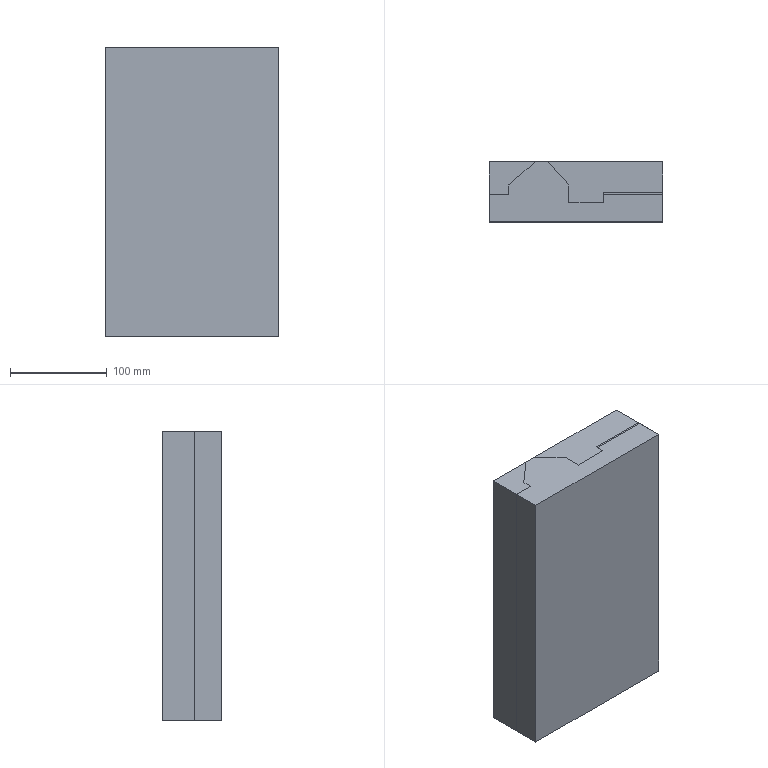Part | NX | 3 solids | 34 faces | box 180 x 62 x 300 mm | volume 7148100 mm3 | plane 34
STEP:
#1=CARTESIAN_POINT('',(-90.,31.,300.));
#2=VERTEX_POINT('',#1);
#3=CARTESIAN_POINT('',(-90.,31.,0.));
#4=VERTEX_POINT('',#3);
#5=CARTESIAN_POINT('',(-90.,31.,150.));
#6=DIRECTION('',(0.,0.,-1.));
#7=VECTOR('',#6,1000.);
#8=LINE('',#5,#7);
#9=EDGE_CURVE('',#2,#4,#8,.T.);
#10=ORIENTED_EDGE('',*,*,#9,.F.);
#11=CARTESIAN_POINT('',(90.,31.,300.));
#12=VERTEX_POINT('',#11);
#13=CARTESIAN_POINT('',(0.,31.,300.));
#14=DIRECTION('',(-1.,0.,0.));
#15=VECTOR('',#14,1000.);
#16=LINE('',#13,#15);
#17=EDGE_CURVE('',#12,#2,#16,.T.);
#18=ORIENTED_EDGE('',*,*,#17,.F.);
#19=CARTESIAN_POINT('',(90.,31.,0.));
#20=VERTEX_POINT('',#19);
#21=CARTESIAN_POINT('',(90.,31.,150.));
#22=DIRECTION('',(0.,0.,1.));
#23=VECTOR('',#22,1000.);
#24=LINE('',#21,#23);
#25=EDGE_CURVE('',#20,#12,#24,.T.);
#26=ORIENTED_EDGE('',*,*,#25,.F.);
#27=CARTESIAN_POINT('',(0.,31.,0.));
#28=DIRECTION('',(1.,0.,0.));
#29=VECTOR('',#28,1000.);
#30=LINE('',#27,#29);
#31=EDGE_CURVE('',#4,#20,#30,.T.);
#32=ORIENTED_EDGE('',*,*,#31,.F.);
#33=EDGE_LOOP('',(#10,#18,#26,#32));
#34=FACE_BOUND('',#33,.T.);
#35=CARTESIAN_POINT('',(0.,31.,150.));
#36=DIRECTION('',(0.,1.,0.));
#37=DIRECTION('',(0.,0.,1.));
#38=AXIS2_PLACEMENT_3D('',#35,#36,#37);
#39=PLANE('',#38);
#40=ADVANCED_FACE('',(#34),#39,.T.);
#41=CARTESIAN_POINT('',(-90.,-31.,300.));
#42=VERTEX_POINT('',#41);
#43=CARTESIAN_POINT('',(-90.,-31.,300.));
#44=DIRECTION('',(0.,1.,0.));
#45=VECTOR('',#44,1000.);
#46=LINE('',#43,#45);
#47=EDGE_CURVE('',#42,#2,#46,.T.);
#48=ORIENTED_EDGE('',*,*,#47,.T.);
#49=ORIENTED_EDGE('',*,*,#9,.T.);
#50=CARTESIAN_POINT('',(-90.,-31.,0.));
#51=VERTEX_POINT('',#50);
#52=CARTESIAN_POINT('',(-90.,-31.,0.));
#53=DIRECTION('',(0.,1.,0.));
#54=VECTOR('',#53,1000.);
#55=LINE('',#52,#54);
#56=EDGE_CURVE('',#51,#4,#55,.T.);
#57=ORIENTED_EDGE('',*,*,#56,.F.);
#58=CARTESIAN_POINT('',(-90.,-31.,150.));
#59=DIRECTION('',(0.,0.,1.));
#60=VECTOR('',#59,1000.);
#61=LINE('',#58,#60);
#62=EDGE_CURVE('',#51,#42,#61,.T.);
#63=ORIENTED_EDGE('',*,*,#62,.T.);
#64=EDGE_LOOP('',(#48,#49,#57,#63));
#65=FACE_BOUND('',#64,.T.);
#66=CARTESIAN_POINT('',(-90.,-31.,150.));
#67=DIRECTION('',(-1.,0.,0.));
#68=DIRECTION('',(0.,-1.,0.));
#69=AXIS2_PLACEMENT_3D('',#66,#67,#68);
#70=PLANE('',#69);
#71=ADVANCED_FACE('',(#65),#70,.T.);
#72=ORIENTED_EDGE('',*,*,#56,.T.);
#73=ORIENTED_EDGE('',*,*,#31,.T.);
#74=CARTESIAN_POINT('',(90.,-31.,0.));
#75=VERTEX_POINT('',#74);
#76=CARTESIAN_POINT('',(90.,-31.,0.));
#77=DIRECTION('',(0.,1.,0.));
#78=VECTOR('',#77,1000.);
#79=LINE('',#76,#78);
#80=EDGE_CURVE('',#75,#20,#79,.T.);
#81=ORIENTED_EDGE('',*,*,#80,.F.);
#82=CARTESIAN_POINT('',(0.,-31.,0.));
#83=DIRECTION('',(-1.,0.,0.));
#84=VECTOR('',#83,1000.);
#85=LINE('',#82,#84);
#86=EDGE_CURVE('',#75,#51,#85,.T.);
#87=ORIENTED_EDGE('',*,*,#86,.T.);
#88=EDGE_LOOP('',(#72,#73,#81,#87));
#89=FACE_BOUND('',#88,.T.);
#90=CARTESIAN_POINT('',(0.,-31.,0.));
#91=DIRECTION('',(0.,0.,-1.));
#92=DIRECTION('',(0.,1.,0.));
#93=AXIS2_PLACEMENT_3D('',#90,#91,#92);
#94=PLANE('',#93);
#95=ADVANCED_FACE('',(#89),#94,.T.);
#96=ORIENTED_EDGE('',*,*,#80,.T.);
#97=ORIENTED_EDGE('',*,*,#25,.T.);
#98=CARTESIAN_POINT('',(90.,-31.,300.));
#99=VERTEX_POINT('',#98);
#100=CARTESIAN_POINT('',(90.,-31.,300.));
#101=DIRECTION('',(0.,1.,0.));
#102=VECTOR('',#101,1000.);
#103=LINE('',#100,#102);
#104=EDGE_CURVE('',#99,#12,#103,.T.);
#105=ORIENTED_EDGE('',*,*,#104,.F.);
#106=CARTESIAN_POINT('',(90.,-31.,150.));
#107=DIRECTION('',(0.,0.,-1.));
#108=VECTOR('',#107,1000.);
#109=LINE('',#106,#108);
#110=EDGE_CURVE('',#99,#75,#109,.T.);
#111=ORIENTED_EDGE('',*,*,#110,.T.);
#112=EDGE_LOOP('',(#96,#97,#105,#111));
#113=FACE_BOUND('',#112,.T.);
#114=CARTESIAN_POINT('',(90.,-31.,150.));
#115=DIRECTION('',(1.,0.,0.));
#116=DIRECTION('',(0.,1.,0.));
#117=AXIS2_PLACEMENT_3D('',#114,#115,#116);
#118=PLANE('',#117);
#119=ADVANCED_FACE('',(#113),#118,.T.);
#120=CARTESIAN_POINT('',(0.,-31.,300.));
#121=DIRECTION('',(1.,0.,0.));
#122=VECTOR('',#121,1000.);
#123=LINE('',#120,#122);
#124=EDGE_CURVE('',#42,#99,#123,.T.);
#125=ORIENTED_EDGE('',*,*,#124,.F.);
#126=ORIENTED_EDGE('',*,*,#62,.F.);
#127=ORIENTED_EDGE('',*,*,#86,.F.);
#128=ORIENTED_EDGE('',*,*,#110,.F.);
#129=EDGE_LOOP('',(#125,#126,#127,#128));
#130=FACE_BOUND('',#129,.T.);
#131=CARTESIAN_POINT('',(0.,-31.,150.));
#132=DIRECTION('',(0.,-1.,0.));
#133=DIRECTION('',(0.,0.,-1.));
#134=AXIS2_PLACEMENT_3D('',#131,#132,#133);
#135=PLANE('',#134);
#136=ADVANCED_FACE('',(#130),#135,.T.);
#137=ORIENTED_EDGE('',*,*,#124,.T.);
#138=ORIENTED_EDGE('',*,*,#104,.T.);
#139=ORIENTED_EDGE('',*,*,#17,.T.);
#140=ORIENTED_EDGE('',*,*,#47,.F.);
#141=EDGE_LOOP('',(#137,#138,#139,#140));
#142=FACE_BOUND('',#141,.T.);
#143=CARTESIAN_POINT('',(0.,-31.,300.));
#144=DIRECTION('',(0.,0.,1.));
#145=DIRECTION('',(0.,-1.,0.));
#146=AXIS2_PLACEMENT_3D('',#143,#144,#145);
#147=PLANE('',#146);
#148=ADVANCED_FACE('',(#142),#147,.T.);
#149=CLOSED_SHELL('',(#40,#71,#95,#119,#136,#148));
#150=MANIFOLD_SOLID_BREP('',#149);
#151=CARTESIAN_POINT('',(-69.5,7.,0.));
#152=VERTEX_POINT('',#151);
#153=CARTESIAN_POINT('',(-42.372,31.,0.));
#154=VERTEX_POINT('',#153);
#155=CARTESIAN_POINT('',(-69.5,7.,0.));
#156=DIRECTION('',(0.749,0.6626,0.));
#157=VECTOR('',#156,1000.);
#158=LINE('',#155,#157);
#159=EDGE_CURVE('',#152,#154,#158,.T.);
#160=ORIENTED_EDGE('',*,*,#159,.F.);
#161=CARTESIAN_POINT('',(-69.5,7.,300.));
#162=VERTEX_POINT('',#161);
#163=CARTESIAN_POINT('',(-69.5,7.,300.));
#164=DIRECTION('',(0.,0.,-1.));
#165=VECTOR('',#164,1000.);
#166=LINE('',#163,#165);
#167=EDGE_CURVE('',#162,#152,#166,.T.);
#168=ORIENTED_EDGE('',*,*,#167,.F.);
#169=CARTESIAN_POINT('',(-42.372,31.,300.));
#170=VERTEX_POINT('',#169);
#171=CARTESIAN_POINT('',(-69.5,7.,300.));
#172=DIRECTION('',(0.749,0.6626,0.));
#173=VECTOR('',#172,1000.);
#174=LINE('',#171,#173);
#175=EDGE_CURVE('',#162,#170,#174,.T.);
#176=ORIENTED_EDGE('',*,*,#175,.T.);
#177=CARTESIAN_POINT('',(-42.372,31.,300.));
#178=DIRECTION('',(0.,0.,-1.));
#179=VECTOR('',#178,1000.);
#180=LINE('',#177,#179);
#181=EDGE_CURVE('',#170,#154,#180,.T.);
#182=ORIENTED_EDGE('',*,*,#181,.T.);
#183=EDGE_LOOP('',(#160,#168,#176,#182));
#184=FACE_BOUND('',#183,.T.);
#185=CARTESIAN_POINT('',(-69.5,7.,300.));
#186=DIRECTION('',(-0.6626,0.749,0.));
#187=DIRECTION('',(-0.749,-0.6626,0.));
#188=AXIS2_PLACEMENT_3D('',#185,#186,#187);
#189=PLANE('',#188);
#190=ADVANCED_FACE('',(#184),#189,.T.);
#191=CARTESIAN_POINT('',(-29.372,31.,0.));
#192=VERTEX_POINT('',#191);
#193=CARTESIAN_POINT('',(-42.372,31.,0.));
#194=DIRECTION('',(1.,0.,0.));
#195=VECTOR('',#194,1000.);
#196=LINE('',#193,#195);
#197=EDGE_CURVE('',#154,#192,#196,.T.);
#198=ORIENTED_EDGE('',*,*,#197,.F.);
#199=ORIENTED_EDGE('',*,*,#181,.F.);
#200=CARTESIAN_POINT('',(-29.372,31.,300.));
#201=VERTEX_POINT('',#200);
#202=CARTESIAN_POINT('',(-42.372,31.,300.));
#203=DIRECTION('',(1.,0.,0.));
#204=VECTOR('',#203,1000.);
#205=LINE('',#202,#204);
#206=EDGE_CURVE('',#170,#201,#205,.T.);
#207=ORIENTED_EDGE('',*,*,#206,.T.);
#208=CARTESIAN_POINT('',(-29.372,31.,300.));
#209=DIRECTION('',(0.,0.,-1.));
#210=VECTOR('',#209,1000.);
#211=LINE('',#208,#210);
#212=EDGE_CURVE('',#201,#192,#211,.T.);
#213=ORIENTED_EDGE('',*,*,#212,.T.);
#214=EDGE_LOOP('',(#198,#199,#207,#213));
#215=FACE_BOUND('',#214,.T.);
#216=CARTESIAN_POINT('',(-42.372,31.,300.));
#217=DIRECTION('',(0.,1.,0.));
#218=DIRECTION('',(0.,0.,1.));
#219=AXIS2_PLACEMENT_3D('',#216,#217,#218);
#220=PLANE('',#219);
#221=ADVANCED_FACE('',(#215),#220,.T.);
#222=CARTESIAN_POINT('',(-7.5,7.,0.));
#223=VERTEX_POINT('',#222);
#224=CARTESIAN_POINT('',(-29.372,31.,0.));
#225=DIRECTION('',(0.6736,-0.7391,0.));
#226=VECTOR('',#225,1000.);
#227=LINE('',#224,#226);
#228=EDGE_CURVE('',#192,#223,#227,.T.);
#229=ORIENTED_EDGE('',*,*,#228,.F.);
#230=ORIENTED_EDGE('',*,*,#212,.F.);
#231=CARTESIAN_POINT('',(-7.5,7.,300.));
#232=VERTEX_POINT('',#231);
#233=CARTESIAN_POINT('',(-29.372,31.,300.));
#234=DIRECTION('',(0.6736,-0.7391,0.));
#235=VECTOR('',#234,1000.);
#236=LINE('',#233,#235);
#237=EDGE_CURVE('',#201,#232,#236,.T.);
#238=ORIENTED_EDGE('',*,*,#237,.T.);
#239=CARTESIAN_POINT('',(-7.5,7.,300.));
#240=DIRECTION('',(0.,0.,-1.));
#241=VECTOR('',#240,1000.);
#242=LINE('',#239,#241);
#243=EDGE_CURVE('',#232,#223,#242,.T.);
#244=ORIENTED_EDGE('',*,*,#243,.T.);
#245=EDGE_LOOP('',(#229,#230,#238,#244));
#246=FACE_BOUND('',#245,.T.);
#247=CARTESIAN_POINT('',(-29.372,31.,300.));
#248=DIRECTION('',(0.7391,0.6736,0.));
#249=DIRECTION('',(-0.6736,0.7391,0.));
#250=AXIS2_PLACEMENT_3D('',#247,#248,#249);
#251=PLANE('',#250);
#252=ADVANCED_FACE('',(#246),#251,.T.);
#253=CARTESIAN_POINT('',(-7.5,-11.,0.));
#254=VERTEX_POINT('',#253);
#255=CARTESIAN_POINT('',(-7.5,-3.,0.));
#256=DIRECTION('',(0.,-1.,0.));
#257=VECTOR('',#256,1000.);
#258=LINE('',#255,#257);
#259=EDGE_CURVE('',#223,#254,#258,.T.);
#260=ORIENTED_EDGE('',*,*,#259,.F.);
#261=ORIENTED_EDGE('',*,*,#243,.F.);
#262=CARTESIAN_POINT('',(-7.5,-11.,300.));
#263=VERTEX_POINT('',#262);
#264=CARTESIAN_POINT('',(-7.5,7.,300.));
#265=DIRECTION('',(0.,-1.,0.));
#266=VECTOR('',#265,1000.);
#267=LINE('',#264,#266);
#268=EDGE_CURVE('',#232,#263,#267,.T.);
#269=ORIENTED_EDGE('',*,*,#268,.T.);
#270=CARTESIAN_POINT('',(-7.5,-11.,300.));
#271=DIRECTION('',(0.,0.,-1.));
#272=VECTOR('',#271,1000.);
#273=LINE('',#270,#272);
#274=EDGE_CURVE('',#263,#254,#273,.T.);
#275=ORIENTED_EDGE('',*,*,#274,.T.);
#276=EDGE_LOOP('',(#260,#261,#269,#275));
#277=FACE_BOUND('',#276,.T.);
#278=CARTESIAN_POINT('',(-7.5,-3.,300.));
#279=DIRECTION('',(1.,0.,0.));
#280=DIRECTION('',(0.,0.,-1.));
#281=AXIS2_PLACEMENT_3D('',#278,#279,#280);
#282=PLANE('',#281);
#283=ADVANCED_FACE('',(#277),#282,.T.);
#284=CARTESIAN_POINT('',(28.5,-11.,0.));
#285=VERTEX_POINT('',#284);
#286=CARTESIAN_POINT('',(-7.5,-11.,0.));
#287=DIRECTION('',(1.,0.,0.));
#288=VECTOR('',#287,1000.);
#289=LINE('',#286,#288);
#290=EDGE_CURVE('',#254,#285,#289,.T.);
#291=ORIENTED_EDGE('',*,*,#290,.F.);
#292=ORIENTED_EDGE('',*,*,#274,.F.);
#293=CARTESIAN_POINT('',(28.5,-11.,300.));
#294=VERTEX_POINT('',#293);
#295=CARTESIAN_POINT('',(-7.5,-11.,300.));
#296=DIRECTION('',(1.,0.,0.));
#297=VECTOR('',#296,1000.);
#298=LINE('',#295,#297);
#299=EDGE_CURVE('',#263,#294,#298,.T.);
#300=ORIENTED_EDGE('',*,*,#299,.T.);
#301=CARTESIAN_POINT('',(28.5,-11.,300.));
#302=DIRECTION('',(0.,0.,-1.));
#303=VECTOR('',#302,1000.);
#304=LINE('',#301,#303);
#305=EDGE_CURVE('',#294,#285,#304,.T.);
#306=ORIENTED_EDGE('',*,*,#305,.T.);
#307=EDGE_LOOP('',(#291,#292,#300,#306));
#308=FACE_BOUND('',#307,.T.);
#309=CARTESIAN_POINT('',(-7.5,-11.,300.));
#310=DIRECTION('',(0.,1.,0.));
#311=DIRECTION('',(-1.,0.,0.));
#312=AXIS2_PLACEMENT_3D('',#309,#310,#311);
#313=PLANE('',#312);
#314=ADVANCED_FACE('',(#308),#313,.T.);
#315=CARTESIAN_POINT('',(28.5,-1.,0.));
#316=VERTEX_POINT('',#315);
#317=CARTESIAN_POINT('',(28.5,-11.,0.));
#318=DIRECTION('',(0.,1.,0.));
#319=VECTOR('',#318,1000.);
#320=LINE('',#317,#319);
#321=EDGE_CURVE('',#285,#316,#320,.T.);
#322=ORIENTED_EDGE('',*,*,#321,.F.);
#323=ORIENTED_EDGE('',*,*,#305,.F.);
#324=CARTESIAN_POINT('',(28.5,-1.,300.));
#325=VERTEX_POINT('',#324);
#326=CARTESIAN_POINT('',(28.5,-11.,300.));
#327=DIRECTION('',(0.,1.,0.));
#328=VECTOR('',#327,1000.);
#329=LINE('',#326,#328);
#330=EDGE_CURVE('',#294,#325,#329,.T.);
#331=ORIENTED_EDGE('',*,*,#330,.T.);
#332=CARTESIAN_POINT('',(28.5,-1.,300.));
#333=DIRECTION('',(0.,0.,-1.));
#334=VECTOR('',#333,1000.);
#335=LINE('',#332,#334);
#336=EDGE_CURVE('',#325,#316,#335,.T.);
#337=ORIENTED_EDGE('',*,*,#336,.T.);
#338=EDGE_LOOP('',(#322,#323,#331,#337));
#339=FACE_BOUND('',#338,.T.);
#340=CARTESIAN_POINT('',(28.5,-11.,300.));
#341=DIRECTION('',(-1.,0.,0.));
#342=DIRECTION('',(0.,0.,1.));
#343=AXIS2_PLACEMENT_3D('',#340,#341,#342);
#344=PLANE('',#343);
#345=ADVANCED_FACE('',(#339),#344,.T.);
#346=CARTESIAN_POINT('',(90.,-1.,0.));
#347=VERTEX_POINT('',#346);
#348=CARTESIAN_POINT('',(0.,-1.,0.));
#349=DIRECTION('',(1.,0.,0.));
#350=VECTOR('',#349,1000.);
#351=LINE('',#348,#350);
#352=EDGE_CURVE('',#316,#347,#351,.T.);
#353=ORIENTED_EDGE('',*,*,#352,.F.);
#354=ORIENTED_EDGE('',*,*,#336,.F.);
#355=CARTESIAN_POINT('',(90.,-1.,300.));
#356=VERTEX_POINT('',#355);
#357=CARTESIAN_POINT('',(0.,-1.,300.));
#358=DIRECTION('',(1.,0.,0.));
#359=VECTOR('',#358,1000.);
#360=LINE('',#357,#359);
#361=EDGE_CURVE('',#325,#356,#360,.T.);
#362=ORIENTED_EDGE('',*,*,#361,.T.);
#363=CARTESIAN_POINT('',(90.,-1.,300.));
#364=DIRECTION('',(0.,0.,-1.));
#365=VECTOR('',#364,1000.);
#366=LINE('',#363,#365);
#367=EDGE_CURVE('',#356,#347,#366,.T.);
#368=ORIENTED_EDGE('',*,*,#367,.T.);
#369=EDGE_LOOP('',(#353,#354,#362,#368));
#370=FACE_BOUND('',#369,.T.);
#371=CARTESIAN_POINT('',(28.5,-1.,300.));
#372=DIRECTION('',(0.,1.,0.));
#373=DIRECTION('',(-1.,0.,0.));
#374=AXIS2_PLACEMENT_3D('',#371,#372,#373);
#375=PLANE('',#374);
#376=ADVANCED_FACE('',(#370),#375,.T.);
#377=CARTESIAN_POINT('',(90.,-31.,0.));
#378=VERTEX_POINT('',#377);
#379=CARTESIAN_POINT('',(90.,0.,0.));
#380=DIRECTION('',(0.,-1.,0.));
#381=VECTOR('',#380,1000.);
#382=LINE('',#379,#381);
#383=EDGE_CURVE('',#347,#378,#382,.T.);
#384=ORIENTED_EDGE('',*,*,#383,.F.);
#385=ORIENTED_EDGE('',*,*,#367,.F.);
#386=CARTESIAN_POINT('',(90.,-31.,300.));
#387=VERTEX_POINT('',#386);
#388=CARTESIAN_POINT('',(90.,0.,300.));
#389=DIRECTION('',(0.,-1.,0.));
#390=VECTOR('',#389,1000.);
#391=LINE('',#388,#390);
#392=EDGE_CURVE('',#356,#387,#391,.T.);
#393=ORIENTED_EDGE('',*,*,#392,.T.);
#394=CARTESIAN_POINT('',(90.,-31.,300.));
#395=DIRECTION('',(0.,0.,-1.));
#396=VECTOR('',#395,1000.);
#397=LINE('',#394,#396);
#398=EDGE_CURVE('',#387,#378,#397,.T.);
#399=ORIENTED_EDGE('',*,*,#398,.T.);
#400=EDGE_LOOP('',(#384,#385,#393,#399));
#401=FACE_BOUND('',#400,.T.);
#402=CARTESIAN_POINT('',(90.,-3.,300.));
#403=DIRECTION('',(1.,0.,0.));
#404=DIRECTION('',(0.,1.,0.));
#405=AXIS2_PLACEMENT_3D('',#402,#403,#404);
#406=PLANE('',#405);
#407=ADVANCED_FACE('',(#401),#406,.T.);
#408=CARTESIAN_POINT('',(-90.,-31.,0.));
#409=VERTEX_POINT('',#408);
#410=CARTESIAN_POINT('',(90.5,-31.,0.));
#411=DIRECTION('',(-1.,0.,0.));
#412=VECTOR('',#411,1000.);
#413=LINE('',#410,#412);
#414=EDGE_CURVE('',#378,#409,#413,.T.);
#415=ORIENTED_EDGE('',*,*,#414,.F.);
#416=ORIENTED_EDGE('',*,*,#398,.F.);
#417=CARTESIAN_POINT('',(-90.,-31.,300.));
#418=VERTEX_POINT('',#417);
#419=CARTESIAN_POINT('',(90.5,-31.,300.));
#420=DIRECTION('',(-1.,0.,0.));
#421=VECTOR('',#420,1000.);
#422=LINE('',#419,#421);
#423=EDGE_CURVE('',#387,#418,#422,.T.);
#424=ORIENTED_EDGE('',*,*,#423,.T.);
#425=CARTESIAN_POINT('',(-90.,-31.,300.));
#426=DIRECTION('',(0.,0.,-1.));
#427=VECTOR('',#426,1000.);
#428=LINE('',#425,#427);
#429=EDGE_CURVE('',#418,#409,#428,.T.);
#430=ORIENTED_EDGE('',*,*,#429,.T.);
#431=EDGE_LOOP('',(#415,#416,#424,#430));
#432=FACE_BOUND('',#431,.T.);
#433=CARTESIAN_POINT('',(90.5,-31.,300.));
#434=DIRECTION('',(0.,-1.,0.));
#435=DIRECTION('',(0.,0.,-1.));
#436=AXIS2_PLACEMENT_3D('',#433,#434,#435);
#437=PLANE('',#436);
#438=ADVANCED_FACE('',(#432),#437,.T.);
#439=CARTESIAN_POINT('',(-90.,-3.,0.));
#440=VERTEX_POINT('',#439);
#441=CARTESIAN_POINT('',(-90.,0.,0.));
#442=DIRECTION('',(0.,1.,0.));
#443=VECTOR('',#442,1000.);
#444=LINE('',#441,#443);
#445=EDGE_CURVE('',#409,#440,#444,.T.);
#446=ORIENTED_EDGE('',*,*,#445,.F.);
#447=ORIENTED_EDGE('',*,*,#429,.F.);
#448=CARTESIAN_POINT('',(-90.,-3.,300.));
#449=VERTEX_POINT('',#448);
#450=CARTESIAN_POINT('',(-90.,0.,300.));
#451=DIRECTION('',(0.,1.,0.));
#452=VECTOR('',#451,1000.);
#453=LINE('',#450,#452);
#454=EDGE_CURVE('',#418,#449,#453,.T.);
#455=ORIENTED_EDGE('',*,*,#454,.T.);
#456=CARTESIAN_POINT('',(-90.,-3.,300.));
#457=DIRECTION('',(0.,0.,-1.));
#458=VECTOR('',#457,1000.);
#459=LINE('',#456,#458);
#460=EDGE_CURVE('',#449,#440,#459,.T.);
#461=ORIENTED_EDGE('',*,*,#460,.T.);
#462=EDGE_LOOP('',(#446,#447,#455,#461));
#463=FACE_BOUND('',#462,.T.);
#464=CARTESIAN_POINT('',(-90.,-31.,300.));
#465=DIRECTION('',(-1.,0.,0.));
#466=DIRECTION('',(0.,-1.,0.));
#467=AXIS2_PLACEMENT_3D('',#464,#465,#466);
#468=PLANE('',#467);
#469=ADVANCED_FACE('',(#463),#468,.T.);
#470=CARTESIAN_POINT('',(-69.5,-3.,0.));
#471=VERTEX_POINT('',#470);
#472=CARTESIAN_POINT('',(-90.5,-3.,0.));
#473=DIRECTION('',(1.,0.,0.));
#474=VECTOR('',#473,1000.);
#475=LINE('',#472,#474);
#476=EDGE_CURVE('',#440,#471,#475,.T.);
#477=ORIENTED_EDGE('',*,*,#476,.F.);
#478=ORIENTED_EDGE('',*,*,#460,.F.);
#479=CARTESIAN_POINT('',(-69.5,-3.,300.));
#480=VERTEX_POINT('',#479);
#481=CARTESIAN_POINT('',(-90.5,-3.,300.));
#482=DIRECTION('',(1.,0.,0.));
#483=VECTOR('',#482,1000.);
#484=LINE('',#481,#483);
#485=EDGE_CURVE('',#449,#480,#484,.T.);
#486=ORIENTED_EDGE('',*,*,#485,.T.);
#487=CARTESIAN_POINT('',(-69.5,-3.,300.));
#488=DIRECTION('',(0.,0.,-1.));
#489=VECTOR('',#488,1000.);
#490=LINE('',#487,#489);
#491=EDGE_CURVE('',#480,#471,#490,.T.);
#492=ORIENTED_EDGE('',*,*,#491,.T.);
#493=EDGE_LOOP('',(#477,#478,#486,#492));
#494=FACE_BOUND('',#493,.T.);
#495=CARTESIAN_POINT('',(-90.5,-3.,300.));
#496=DIRECTION('',(0.,1.,0.));
#497=DIRECTION('',(0.,0.,1.));
#498=AXIS2_PLACEMENT_3D('',#495,#496,#497);
#499=PLANE('',#498);
#500=ADVANCED_FACE('',(#494),#499,.T.);
#501=CARTESIAN_POINT('',(-69.5,-3.,0.));
#502=DIRECTION('',(0.,1.,0.));
#503=VECTOR('',#502,1000.);
#504=LINE('',#501,#503);
#505=EDGE_CURVE('',#471,#152,#504,.T.);
#506=ORIENTED_EDGE('',*,*,#505,.F.);
#507=ORIENTED_EDGE('',*,*,#491,.F.);
#508=CARTESIAN_POINT('',(-69.5,-3.,300.));
#509=DIRECTION('',(0.,1.,0.));
#510=VECTOR('',#509,1000.);
#511=LINE('',#508,#510);
#512=EDGE_CURVE('',#480,#162,#511,.T.);
#513=ORIENTED_EDGE('',*,*,#512,.T.);
#514=ORIENTED_EDGE('',*,*,#167,.T.);
#515=EDGE_LOOP('',(#506,#507,#513,#514));
#516=FACE_BOUND('',#515,.T.);
#517=CARTESIAN_POINT('',(-69.5,-3.,300.));
#518=DIRECTION('',(-1.,0.,0.));
#519=DIRECTION('',(0.,0.,1.));
#520=AXIS2_PLACEMENT_3D('',#517,#518,#519);
#521=PLANE('',#520);
#522=ADVANCED_FACE('',(#516),#521,.T.);
#523=ORIENTED_EDGE('',*,*,#175,.F.);
#524=ORIENTED_EDGE('',*,*,#512,.F.);
#525=ORIENTED_EDGE('',*,*,#485,.F.);
#526=ORIENTED_EDGE('',*,*,#454,.F.);
#527=ORIENTED_EDGE('',*,*,#423,.F.);
#528=ORIENTED_EDGE('',*,*,#392,.F.);
#529=ORIENTED_EDGE('',*,*,#361,.F.);
#530=ORIENTED_EDGE('',*,*,#330,.F.);
#531=ORIENTED_EDGE('',*,*,#299,.F.);
#532=ORIENTED_EDGE('',*,*,#268,.F.);
#533=ORIENTED_EDGE('',*,*,#237,.F.);
#534=ORIENTED_EDGE('',*,*,#206,.F.);
#535=EDGE_LOOP('',(#523,#524,#525,#526,#527,#528,#529,#530,#531,#532,#533,#534));
#536=FACE_BOUND('',#535,.T.);
#537=CARTESIAN_POINT('',(0.,0.,300.));
#538=DIRECTION('',(0.,0.,-1.));
#539=DIRECTION('',(-1.,0.,0.));
#540=AXIS2_PLACEMENT_3D('',#537,#538,#539);
#541=PLANE('',#540);
#542=ADVANCED_FACE('',(#536),#541,.F.);
#543=ORIENTED_EDGE('',*,*,#159,.T.);
#544=ORIENTED_EDGE('',*,*,#197,.T.);
#545=ORIENTED_EDGE('',*,*,#228,.T.);
#546=ORIENTED_EDGE('',*,*,#259,.T.);
#547=ORIENTED_EDGE('',*,*,#290,.T.);
#548=ORIENTED_EDGE('',*,*,#321,.T.);
#549=ORIENTED_EDGE('',*,*,#352,.T.);
#550=ORIENTED_EDGE('',*,*,#383,.T.);
#551=ORIENTED_EDGE('',*,*,#414,.T.);
#552=ORIENTED_EDGE('',*,*,#445,.T.);
#553=ORIENTED_EDGE('',*,*,#476,.T.);
#554=ORIENTED_EDGE('',*,*,#505,.T.);
#555=EDGE_LOOP('',(#543,#544,#545,#546,#547,#548,#549,#550,#551,#552,#553,#554));
#556=FACE_BOUND('',#555,.T.);
#557=CARTESIAN_POINT('',(0.,0.,0.));
#558=DIRECTION('',(0.,0.,-1.));
#559=DIRECTION('',(-1.,0.,0.));
#560=AXIS2_PLACEMENT_3D('',#557,#558,#559);
#561=PLANE('',#560);
#562=ADVANCED_FACE('',(#556),#561,.T.);
#563=CLOSED_SHELL('',(#190,#221,#252,#283,#314,#345,#376,#407,#438,#469,#500,#522,#542,#562));
#564=MANIFOLD_SOLID_BREP('',#563);
#565=CARTESIAN_POINT('',(-69.5,7.,0.));
#566=VERTEX_POINT('',#565);
#567=CARTESIAN_POINT('',(-42.372,31.,0.));
#568=VERTEX_POINT('',#567);
#569=CARTESIAN_POINT('',(-69.5,7.,0.));
#570=DIRECTION('',(0.749,0.6626,0.));
#571=VECTOR('',#570,1000.);
#572=LINE('',#569,#571);
#573=EDGE_CURVE('',#566,#568,#572,.T.);
#574=ORIENTED_EDGE('',*,*,#573,.F.);
#575=CARTESIAN_POINT('',(-69.5,7.,300.));
#576=VERTEX_POINT('',#575);
#577=CARTESIAN_POINT('',(-69.5,7.,300.));
#578=DIRECTION('',(0.,0.,-1.));
#579=VECTOR('',#578,1000.);
#580=LINE('',#577,#579);
#581=EDGE_CURVE('',#576,#566,#580,.T.);
#582=ORIENTED_EDGE('',*,*,#581,.F.);
#583=CARTESIAN_POINT('',(-42.372,31.,300.));
#584=VERTEX_POINT('',#583);
#585=CARTESIAN_POINT('',(-69.5,7.,300.));
#586=DIRECTION('',(0.749,0.6626,0.));
#587=VECTOR('',#586,1000.);
#588=LINE('',#585,#587);
#589=EDGE_CURVE('',#576,#584,#588,.T.);
#590=ORIENTED_EDGE('',*,*,#589,.T.);
#591=CARTESIAN_POINT('',(-42.372,31.,300.));
#592=DIRECTION('',(0.,0.,-1.));
#593=VECTOR('',#592,1000.);
#594=LINE('',#591,#593);
#595=EDGE_CURVE('',#584,#568,#594,.T.);
#596=ORIENTED_EDGE('',*,*,#595,.T.);
#597=EDGE_LOOP('',(#574,#582,#590,#596));
#598=FACE_BOUND('',#597,.T.);
#599=CARTESIAN_POINT('',(-69.5,7.,300.));
#600=DIRECTION('',(-0.6626,0.749,0.));
#601=DIRECTION('',(-0.749,-0.6626,0.));
#602=AXIS2_PLACEMENT_3D('',#599,#600,#601);
#603=PLANE('',#602);
#604=ADVANCED_FACE('',(#598),#603,.T.);
#605=CARTESIAN_POINT('',(-29.372,31.,0.));
#606=VERTEX_POINT('',#605);
#607=CARTESIAN_POINT('',(-42.372,31.,0.));
#608=DIRECTION('',(1.,0.,0.));
#609=VECTOR('',#608,1000.);
#610=LINE('',#607,#609);
#611=EDGE_CURVE('',#568,#606,#610,.T.);
#612=ORIENTED_EDGE('',*,*,#611,.F.);
#613=ORIENTED_EDGE('',*,*,#595,.F.);
#614=CARTESIAN_POINT('',(-29.372,31.,300.));
#615=VERTEX_POINT('',#614);
#616=CARTESIAN_POINT('',(-42.372,31.,300.));
#617=DIRECTION('',(1.,0.,0.));
#618=VECTOR('',#617,1000.);
#619=LINE('',#616,#618);
#620=EDGE_CURVE('',#584,#615,#619,.T.);
#621=ORIENTED_EDGE('',*,*,#620,.T.);
#622=CARTESIAN_POINT('',(-29.372,31.,300.));
#623=DIRECTION('',(0.,0.,-1.));
#624=VECTOR('',#623,1000.);
#625=LINE('',#622,#624);
#626=EDGE_CURVE('',#615,#606,#625,.T.);
#627=ORIENTED_EDGE('',*,*,#626,.T.);
#628=EDGE_LOOP('',(#612,#613,#621,#627));
#629=FACE_BOUND('',#628,.T.);
#630=CARTESIAN_POINT('',(-42.372,31.,300.));
#631=DIRECTION('',(0.,1.,0.));
#632=DIRECTION('',(0.,0.,1.));
#633=AXIS2_PLACEMENT_3D('',#630,#631,#632);
#634=PLANE('',#633);
#635=ADVANCED_FACE('',(#629),#634,.T.);
#636=CARTESIAN_POINT('',(-7.5,7.,0.));
#637=VERTEX_POINT('',#636);
#638=CARTESIAN_POINT('',(-29.372,31.,0.));
#639=DIRECTION('',(0.6736,-0.7391,0.));
#640=VECTOR('',#639,1000.);
#641=LINE('',#638,#640);
#642=EDGE_CURVE('',#606,#637,#641,.T.);
#643=ORIENTED_EDGE('',*,*,#642,.F.);
#644=ORIENTED_EDGE('',*,*,#626,.F.);
#645=CARTESIAN_POINT('',(-7.5,7.,300.));
#646=VERTEX_POINT('',#645);
#647=CARTESIAN_POINT('',(-29.372,31.,300.));
#648=DIRECTION('',(0.6736,-0.7391,0.));
#649=VECTOR('',#648,1000.);
#650=LINE('',#647,#649);
#651=EDGE_CURVE('',#615,#646,#650,.T.);
#652=ORIENTED_EDGE('',*,*,#651,.T.);
#653=CARTESIAN_POINT('',(-7.5,7.,300.));
#654=DIRECTION('',(0.,0.,-1.));
#655=VECTOR('',#654,1000.);
#656=LINE('',#653,#655);
#657=EDGE_CURVE('',#646,#637,#656,.T.);
#658=ORIENTED_EDGE('',*,*,#657,.T.);
#659=EDGE_LOOP('',(#643,#644,#652,#658));
#660=FACE_BOUND('',#659,.T.);
#661=CARTESIAN_POINT('',(-29.372,31.,300.));
#662=DIRECTION('',(0.7391,0.6736,0.));
#663=DIRECTION('',(-0.6736,0.7391,0.));
#664=AXIS2_PLACEMENT_3D('',#661,#662,#663);
#665=PLANE('',#664);
#666=ADVANCED_FACE('',(#660),#665,.T.);
#667=CARTESIAN_POINT('',(-7.5,-11.,0.));
#668=VERTEX_POINT('',#667);
#669=CARTESIAN_POINT('',(-7.5,-3.,0.));
#670=DIRECTION('',(0.,-1.,0.));
#671=VECTOR('',#670,1000.);
#672=LINE('',#669,#671);
#673=EDGE_CURVE('',#637,#668,#672,.T.);
#674=ORIENTED_EDGE('',*,*,#673,.F.);
#675=ORIENTED_EDGE('',*,*,#657,.F.);
#676=CARTESIAN_POINT('',(-7.5,-11.,300.));
#677=VERTEX_POINT('',#676);
#678=CARTESIAN_POINT('',(-7.5,7.,300.));
#679=DIRECTION('',(0.,-1.,0.));
#680=VECTOR('',#679,1000.);
#681=LINE('',#678,#680);
#682=EDGE_CURVE('',#646,#677,#681,.T.);
#683=ORIENTED_EDGE('',*,*,#682,.T.);
#684=CARTESIAN_POINT('',(-7.5,-11.,300.));
#685=DIRECTION('',(0.,0.,-1.));
#686=VECTOR('',#685,1000.);
#687=LINE('',#684,#686);
#688=EDGE_CURVE('',#677,#668,#687,.T.);
#689=ORIENTED_EDGE('',*,*,#688,.T.);
#690=EDGE_LOOP('',(#674,#675,#683,#689));
#691=FACE_BOUND('',#690,.T.);
#692=CARTESIAN_POINT('',(-7.5,-3.,300.));
#693=DIRECTION('',(1.,0.,0.));
#694=DIRECTION('',(0.,0.,-1.));
#695=AXIS2_PLACEMENT_3D('',#692,#693,#694);
#696=PLANE('',#695);
#697=ADVANCED_FACE('',(#691),#696,.T.);
#698=CARTESIAN_POINT('',(28.5,-11.,0.));
#699=VERTEX_POINT('',#698);
#700=CARTESIAN_POINT('',(-7.5,-11.,0.));
#701=DIRECTION('',(1.,0.,0.));
#702=VECTOR('',#701,1000.);
#703=LINE('',#700,#702);
#704=EDGE_CURVE('',#668,#699,#703,.T.);
#705=ORIENTED_EDGE('',*,*,#704,.F.);
#706=ORIENTED_EDGE('',*,*,#688,.F.);
#707=CARTESIAN_POINT('',(28.5,-11.,300.));
#708=VERTEX_POINT('',#707);
#709=CARTESIAN_POINT('',(-7.5,-11.,300.));
#710=DIRECTION('',(1.,0.,0.));
#711=VECTOR('',#710,1000.);
#712=LINE('',#709,#711);
#713=EDGE_CURVE('',#677,#708,#712,.T.);
#714=ORIENTED_EDGE('',*,*,#713,.T.);
#715=CARTESIAN_POINT('',(28.5,-11.,300.));
#716=DIRECTION('',(0.,0.,-1.));
#717=VECTOR('',#716,1000.);
#718=LINE('',#715,#717);
#719=EDGE_CURVE('',#708,#699,#718,.T.);
#720=ORIENTED_EDGE('',*,*,#719,.T.);
#721=EDGE_LOOP('',(#705,#706,#714,#720));
#722=FACE_BOUND('',#721,.T.);
#723=CARTESIAN_POINT('',(-7.5,-11.,300.));
#724=DIRECTION('',(0.,1.,0.));
#725=DIRECTION('',(-1.,0.,0.));
#726=AXIS2_PLACEMENT_3D('',#723,#724,#725);
#727=PLANE('',#726);
#728=ADVANCED_FACE('',(#722),#727,.T.);
#729=CARTESIAN_POINT('',(28.5,-3.,0.));
#730=VERTEX_POINT('',#729);
#731=CARTESIAN_POINT('',(28.5,-11.,0.));
#732=DIRECTION('',(0.,1.,0.));
#733=VECTOR('',#732,1000.);
#734=LINE('',#731,#733);
#735=EDGE_CURVE('',#699,#730,#734,.T.);
#736=ORIENTED_EDGE('',*,*,#735,.F.);
#737=ORIENTED_EDGE('',*,*,#719,.F.);
#738=CARTESIAN_POINT('',(28.5,-3.,300.));
#739=VERTEX_POINT('',#738);
#740=CARTESIAN_POINT('',(28.5,-11.,300.));
#741=DIRECTION('',(0.,1.,0.));
#742=VECTOR('',#741,1000.);
#743=LINE('',#740,#742);
#744=EDGE_CURVE('',#708,#739,#743,.T.);
#745=ORIENTED_EDGE('',*,*,#744,.T.);
#746=CARTESIAN_POINT('',(28.5,-3.,300.));
#747=DIRECTION('',(0.,0.,-1.));
#748=VECTOR('',#747,1000.);
#749=LINE('',#746,#748);
#750=EDGE_CURVE('',#739,#730,#749,.T.);
#751=ORIENTED_EDGE('',*,*,#750,.T.);
#752=EDGE_LOOP('',(#736,#737,#745,#751));
#753=FACE_BOUND('',#752,.T.);
#754=CARTESIAN_POINT('',(28.5,-11.,300.));
#755=DIRECTION('',(-1.,0.,0.));
#756=DIRECTION('',(0.,0.,1.));
#757=AXIS2_PLACEMENT_3D('',#754,#755,#756);
#758=PLANE('',#757);
#759=ADVANCED_FACE('',(#753),#758,.T.);
#760=CARTESIAN_POINT('',(90.,-3.,0.));
#761=VERTEX_POINT('',#760);
#762=CARTESIAN_POINT('',(28.5,-3.,0.));
#763=DIRECTION('',(1.,0.,0.));
#764=VECTOR('',#763,1000.);
#765=LINE('',#762,#764);
#766=EDGE_CURVE('',#730,#761,#765,.T.);
#767=ORIENTED_EDGE('',*,*,#766,.F.);
#768=ORIENTED_EDGE('',*,*,#750,.F.);
#769=CARTESIAN_POINT('',(90.,-3.,300.));
#770=VERTEX_POINT('',#769);
#771=CARTESIAN_POINT('',(28.5,-3.,300.));
#772=DIRECTION('',(1.,0.,0.));
#773=VECTOR('',#772,1000.);
#774=LINE('',#771,#773);
#775=EDGE_CURVE('',#739,#770,#774,.T.);
#776=ORIENTED_EDGE('',*,*,#775,.T.);
#777=CARTESIAN_POINT('',(90.,-3.,300.));
#778=DIRECTION('',(0.,0.,-1.));
#779=VECTOR('',#778,1000.);
#780=LINE('',#777,#779);
#781=EDGE_CURVE('',#770,#761,#780,.T.);
#782=ORIENTED_EDGE('',*,*,#781,.T.);
#783=EDGE_LOOP('',(#767,#768,#776,#782));
#784=FACE_BOUND('',#783,.T.);
#785=CARTESIAN_POINT('',(28.5,-3.,300.));
#786=DIRECTION('',(0.,1.,0.));
#787=DIRECTION('',(-1.,0.,0.));
#788=AXIS2_PLACEMENT_3D('',#785,#786,#787);
#789=PLANE('',#788);
#790=ADVANCED_FACE('',(#784),#789,.T.);
#791=CARTESIAN_POINT('',(90.,-31.,0.));
#792=VERTEX_POINT('',#791);
#793=CARTESIAN_POINT('',(90.,0.,0.));
#794=DIRECTION('',(0.,-1.,0.));
#795=VECTOR('',#794,1000.);
#796=LINE('',#793,#795);
#797=EDGE_CURVE('',#761,#792,#796,.T.);
#798=ORIENTED_EDGE('',*,*,#797,.F.);
#799=ORIENTED_EDGE('',*,*,#781,.F.);
#800=CARTESIAN_POINT('',(90.,-31.,300.));
#801=VERTEX_POINT('',#800);
#802=CARTESIAN_POINT('',(90.,0.,300.));
#803=DIRECTION('',(0.,-1.,0.));
#804=VECTOR('',#803,1000.);
#805=LINE('',#802,#804);
#806=EDGE_CURVE('',#770,#801,#805,.T.);
#807=ORIENTED_EDGE('',*,*,#806,.T.);
#808=CARTESIAN_POINT('',(90.,-31.,300.));
#809=DIRECTION('',(0.,0.,-1.));
#810=VECTOR('',#809,1000.);
#811=LINE('',#808,#810);
#812=EDGE_CURVE('',#801,#792,#811,.T.);
#813=ORIENTED_EDGE('',*,*,#812,.T.);
#814=EDGE_LOOP('',(#798,#799,#807,#813));
#815=FACE_BOUND('',#814,.T.);
#816=CARTESIAN_POINT('',(90.,-3.,300.));
#817=DIRECTION('',(1.,0.,0.));
#818=DIRECTION('',(0.,1.,0.));
#819=AXIS2_PLACEMENT_3D('',#816,#817,#818);
#820=PLANE('',#819);
#821=ADVANCED_FACE('',(#815),#820,.T.);
#822=CARTESIAN_POINT('',(-90.,-31.,0.));
#823=VERTEX_POINT('',#822);
#824=CARTESIAN_POINT('',(90.5,-31.,0.));
#825=DIRECTION('',(-1.,0.,0.));
#826=VECTOR('',#825,1000.);
#827=LINE('',#824,#826);
#828=EDGE_CURVE('',#792,#823,#827,.T.);
#829=ORIENTED_EDGE('',*,*,#828,.F.);
#830=ORIENTED_EDGE('',*,*,#812,.F.);
#831=CARTESIAN_POINT('',(-90.,-31.,300.));
#832=VERTEX_POINT('',#831);
#833=CARTESIAN_POINT('',(90.5,-31.,300.));
#834=DIRECTION('',(-1.,0.,0.));
#835=VECTOR('',#834,1000.);
#836=LINE('',#833,#835);
#837=EDGE_CURVE('',#801,#832,#836,.T.);
#838=ORIENTED_EDGE('',*,*,#837,.T.);
#839=CARTESIAN_POINT('',(-90.,-31.,300.));
#840=DIRECTION('',(0.,0.,-1.));
#841=VECTOR('',#840,1000.);
#842=LINE('',#839,#841);
#843=EDGE_CURVE('',#832,#823,#842,.T.);
#844=ORIENTED_EDGE('',*,*,#843,.T.);
#845=EDGE_LOOP('',(#829,#830,#838,#844));
#846=FACE_BOUND('',#845,.T.);
#847=CARTESIAN_POINT('',(90.5,-31.,300.));
#848=DIRECTION('',(0.,-1.,0.));
#849=DIRECTION('',(0.,0.,-1.));
#850=AXIS2_PLACEMENT_3D('',#847,#848,#849);
#851=PLANE('',#850);
#852=ADVANCED_FACE('',(#846),#851,.T.);
#853=CARTESIAN_POINT('',(-90.,-3.,0.));
#854=VERTEX_POINT('',#853);
#855=CARTESIAN_POINT('',(-90.,0.,0.));
#856=DIRECTION('',(0.,1.,0.));
#857=VECTOR('',#856,1000.);
#858=LINE('',#855,#857);
#859=EDGE_CURVE('',#823,#854,#858,.T.);
#860=ORIENTED_EDGE('',*,*,#859,.F.);
#861=ORIENTED_EDGE('',*,*,#843,.F.);
#862=CARTESIAN_POINT('',(-90.,-3.,300.));
#863=VERTEX_POINT('',#862);
#864=CARTESIAN_POINT('',(-90.,0.,300.));
#865=DIRECTION('',(0.,1.,0.));
#866=VECTOR('',#865,1000.);
#867=LINE('',#864,#866);
#868=EDGE_CURVE('',#832,#863,#867,.T.);
#869=ORIENTED_EDGE('',*,*,#868,.T.);
#870=CARTESIAN_POINT('',(-90.,-3.,300.));
#871=DIRECTION('',(0.,0.,-1.));
#872=VECTOR('',#871,1000.);
#873=LINE('',#870,#872);
#874=EDGE_CURVE('',#863,#854,#873,.T.);
#875=ORIENTED_EDGE('',*,*,#874,.T.);
#876=EDGE_LOOP('',(#860,#861,#869,#875));
#877=FACE_BOUND('',#876,.T.);
#878=CARTESIAN_POINT('',(-90.,-31.,300.));
#879=DIRECTION('',(-1.,0.,0.));
#880=DIRECTION('',(0.,-1.,0.));
#881=AXIS2_PLACEMENT_3D('',#878,#879,#880);
#882=PLANE('',#881);
#883=ADVANCED_FACE('',(#877),#882,.T.);
#884=CARTESIAN_POINT('',(-69.5,-3.,0.));
#885=VERTEX_POINT('',#884);
#886=CARTESIAN_POINT('',(-90.5,-3.,0.));
#887=DIRECTION('',(1.,0.,0.));
#888=VECTOR('',#887,1000.);
#889=LINE('',#886,#888);
#890=EDGE_CURVE('',#854,#885,#889,.T.);
#891=ORIENTED_EDGE('',*,*,#890,.F.);
#892=ORIENTED_EDGE('',*,*,#874,.F.);
#893=CARTESIAN_POINT('',(-69.5,-3.,300.));
#894=VERTEX_POINT('',#893);
#895=CARTESIAN_POINT('',(-90.5,-3.,300.));
#896=DIRECTION('',(1.,0.,0.));
#897=VECTOR('',#896,1000.);
#898=LINE('',#895,#897);
#899=EDGE_CURVE('',#863,#894,#898,.T.);
#900=ORIENTED_EDGE('',*,*,#899,.T.);
#901=CARTESIAN_POINT('',(-69.5,-3.,300.));
#902=DIRECTION('',(0.,0.,-1.));
#903=VECTOR('',#902,1000.);
#904=LINE('',#901,#903);
#905=EDGE_CURVE('',#894,#885,#904,.T.);
#906=ORIENTED_EDGE('',*,*,#905,.T.);
#907=EDGE_LOOP('',(#891,#892,#900,#906));
#908=FACE_BOUND('',#907,.T.);
#909=CARTESIAN_POINT('',(-90.5,-3.,300.));
#910=DIRECTION('',(0.,1.,0.));
#911=DIRECTION('',(0.,0.,1.));
#912=AXIS2_PLACEMENT_3D('',#909,#910,#911);
#913=PLANE('',#912);
#914=ADVANCED_FACE('',(#908),#913,.T.);
#915=CARTESIAN_POINT('',(-69.5,-3.,0.));
#916=DIRECTION('',(0.,1.,0.));
#917=VECTOR('',#916,1000.);
#918=LINE('',#915,#917);
#919=EDGE_CURVE('',#885,#566,#918,.T.);
#920=ORIENTED_EDGE('',*,*,#919,.F.);
#921=ORIENTED_EDGE('',*,*,#905,.F.);
#922=CARTESIAN_POINT('',(-69.5,-3.,300.));
#923=DIRECTION('',(0.,1.,0.));
#924=VECTOR('',#923,1000.);
#925=LINE('',#922,#924);
#926=EDGE_CURVE('',#894,#576,#925,.T.);
#927=ORIENTED_EDGE('',*,*,#926,.T.);
#928=ORIENTED_EDGE('',*,*,#581,.T.);
#929=EDGE_LOOP('',(#920,#921,#927,#928));
#930=FACE_BOUND('',#929,.T.);
#931=CARTESIAN_POINT('',(-69.5,-3.,300.));
#932=DIRECTION('',(-1.,0.,0.));
#933=DIRECTION('',(0.,0.,1.));
#934=AXIS2_PLACEMENT_3D('',#931,#932,#933);
#935=PLANE('',#934);
#936=ADVANCED_FACE('',(#930),#935,.T.);
#937=ORIENTED_EDGE('',*,*,#589,.F.);
#938=ORIENTED_EDGE('',*,*,#926,.F.);
#939=ORIENTED_EDGE('',*,*,#899,.F.);
#940=ORIENTED_EDGE('',*,*,#868,.F.);
#941=ORIENTED_EDGE('',*,*,#837,.F.);
#942=ORIENTED_EDGE('',*,*,#806,.F.);
#943=ORIENTED_EDGE('',*,*,#775,.F.);
#944=ORIENTED_EDGE('',*,*,#744,.F.);
#945=ORIENTED_EDGE('',*,*,#713,.F.);
#946=ORIENTED_EDGE('',*,*,#682,.F.);
#947=ORIENTED_EDGE('',*,*,#651,.F.);
#948=ORIENTED_EDGE('',*,*,#620,.F.);
#949=EDGE_LOOP('',(#937,#938,#939,#940,#941,#942,#943,#944,#945,#946,#947,#948));
#950=FACE_BOUND('',#949,.T.);
#951=CARTESIAN_POINT('',(0.,0.,300.));
#952=DIRECTION('',(0.,0.,-1.));
#953=DIRECTION('',(-1.,0.,0.));
#954=AXIS2_PLACEMENT_3D('',#951,#952,#953);
#955=PLANE('',#954);
#956=ADVANCED_FACE('',(#950),#955,.F.);
#957=ORIENTED_EDGE('',*,*,#573,.T.);
#958=ORIENTED_EDGE('',*,*,#611,.T.);
#959=ORIENTED_EDGE('',*,*,#642,.T.);
#960=ORIENTED_EDGE('',*,*,#673,.T.);
#961=ORIENTED_EDGE('',*,*,#704,.T.);
#962=ORIENTED_EDGE('',*,*,#735,.T.);
#963=ORIENTED_EDGE('',*,*,#766,.T.);
#964=ORIENTED_EDGE('',*,*,#797,.T.);
#965=ORIENTED_EDGE('',*,*,#828,.T.);
#966=ORIENTED_EDGE('',*,*,#859,.T.);
#967=ORIENTED_EDGE('',*,*,#890,.T.);
#968=ORIENTED_EDGE('',*,*,#919,.T.);
#969=EDGE_LOOP('',(#957,#958,#959,#960,#961,#962,#963,#964,#965,#966,#967,#968));
#970=FACE_BOUND('',#969,.T.);
#971=CARTESIAN_POINT('',(0.,0.,0.));
#972=DIRECTION('',(0.,0.,-1.));
#973=DIRECTION('',(-1.,0.,0.));
#974=AXIS2_PLACEMENT_3D('',#971,#972,#973);
#975=PLANE('',#974);
#976=ADVANCED_FACE('',(#970),#975,.T.);
#977=CLOSED_SHELL('',(#604,#635,#666,#697,#728,#759,#790,#821,#852,#883,#914,#936,#956,#976));
#978=MANIFOLD_SOLID_BREP('',#977);
#979=(LENGTH_UNIT()NAMED_UNIT(*)SI_UNIT(.MILLI.,.METRE.));
#980=UNCERTAINTY_MEASURE_WITH_UNIT(LENGTH_MEASURE(0.00001),#979,'','');
#981=(NAMED_UNIT(*)PLANE_ANGLE_UNIT()SI_UNIT($,.RADIAN.));
#982=(NAMED_UNIT(*)SI_UNIT($,.STERADIAN.)SOLID_ANGLE_UNIT());
#983=(GEOMETRIC_REPRESENTATION_CONTEXT(3)GLOBAL_UNCERTAINTY_ASSIGNED_CONTEXT((#980))GLOBAL_UNIT_ASSIGNED_CONTEXT((#979,#981,#982))REPRESENTATION_CONTEXT('',''));
#984=ADVANCED_BREP_SHAPE_REPRESENTATION('',(#150,#564,#978),#983);